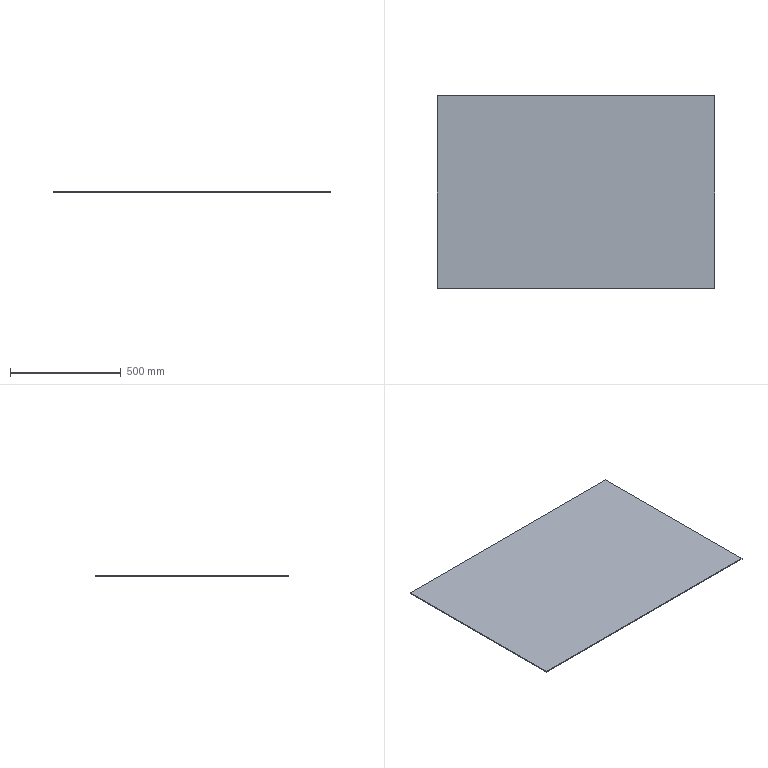Part | STEP file | 08-Middle cover plate | 1 solid | 6 faces | box 1252 x 870 x 4 mm | volume 4356960 mm3 | plane 6
STEP:
#1=CARTESIAN_POINT('',(0.,0.,0.));
#2=DIRECTION('',(0.,0.,1.));
#3=DIRECTION('',(1.,0.,0.));
#4=AXIS2_PLACEMENT_3D('',#1,#2,#3);
#5=CARTESIAN_POINT('',(0.,0.,0.));
#6=VERTEX_POINT('',#5);
#7=CARTESIAN_POINT('',(0.,-870.,0.));
#8=VERTEX_POINT('',#7);
#9=CARTESIAN_POINT('',(0.,0.,0.));
#10=DIRECTION('',(0.,-1.,0.));
#11=VECTOR('',#10,1.);
#12=LINE('',#9,#11);
#13=CARTESIAN_POINT('',(0.,0.,4.));
#14=DIRECTION('',(1.,0.,0.));
#15=DIRECTION('',(0.,1.,0.));
#16=AXIS2_PLACEMENT_3D('',#13,#14,#15);
#17=PLANE('',#16);
#18=CARTESIAN_POINT('',(0.,-4.));
#19=DIRECTION('',(-1.,0.));
#20=VECTOR('',#19,1.);
#21=LINE('',#18,#20);
#22=(GEOMETRIC_REPRESENTATION_CONTEXT(2)PARAMETRIC_REPRESENTATION_CONTEXT()REPRESENTATION_CONTEXT('',''));
#23=DEFINITIONAL_REPRESENTATION('',(#21),#22);
#24=PCURVE('',#17,#23);
#25=CARTESIAN_POINT('',(0.,0.,0.));
#26=DIRECTION('',(0.,0.,1.));
#27=DIRECTION('',(1.,0.,0.));
#28=AXIS2_PLACEMENT_3D('',#25,#26,#27);
#29=PLANE('',#28);
#30=CARTESIAN_POINT('',(0.,0.));
#31=DIRECTION('',(0.,-1.));
#32=VECTOR('',#31,1.);
#33=LINE('',#30,#32);
#34=(GEOMETRIC_REPRESENTATION_CONTEXT(2)PARAMETRIC_REPRESENTATION_CONTEXT()REPRESENTATION_CONTEXT('',''));
#35=DEFINITIONAL_REPRESENTATION('',(#33),#34);
#36=PCURVE('',#29,#35);
#37=SURFACE_CURVE('',#12,(#24,#36),.PCURVE_S1.);
#38=EDGE_CURVE('',#6,#8,#37,.T.);
#39=ORIENTED_EDGE('',*,*,#38,.T.);
#40=CARTESIAN_POINT('',(0.,-870.,4.));
#41=VERTEX_POINT('',#40);
#42=CARTESIAN_POINT('',(0.,-870.,4.));
#43=DIRECTION('',(0.,0.,-1.));
#44=VECTOR('',#43,1.);
#45=LINE('',#42,#44);
#46=CARTESIAN_POINT('',(-870.,0.));
#47=DIRECTION('',(0.,-1.));
#48=VECTOR('',#47,1.);
#49=LINE('',#46,#48);
#50=(GEOMETRIC_REPRESENTATION_CONTEXT(2)PARAMETRIC_REPRESENTATION_CONTEXT()REPRESENTATION_CONTEXT('',''));
#51=DEFINITIONAL_REPRESENTATION('',(#49),#50);
#52=PCURVE('',#17,#51);
#53=CARTESIAN_POINT('',(0.,-870.,4.));
#54=DIRECTION('',(0.,1.,0.));
#55=DIRECTION('',(0.,0.,1.));
#56=AXIS2_PLACEMENT_3D('',#53,#54,#55);
#57=PLANE('',#56);
#58=CARTESIAN_POINT('',(0.,0.));
#59=DIRECTION('',(-1.,0.));
#60=VECTOR('',#59,1.);
#61=LINE('',#58,#60);
#62=(GEOMETRIC_REPRESENTATION_CONTEXT(2)PARAMETRIC_REPRESENTATION_CONTEXT()REPRESENTATION_CONTEXT('',''));
#63=DEFINITIONAL_REPRESENTATION('',(#61),#62);
#64=PCURVE('',#57,#63);
#65=SURFACE_CURVE('',#45,(#52,#64),.PCURVE_S1.);
#66=EDGE_CURVE('',#41,#8,#65,.T.);
#67=ORIENTED_EDGE('',*,*,#66,.F.);
#68=CARTESIAN_POINT('',(0.,0.,4.));
#69=VERTEX_POINT('',#68);
#70=CARTESIAN_POINT('',(0.,0.,4.));
#71=DIRECTION('',(0.,-1.,0.));
#72=VECTOR('',#71,1.);
#73=LINE('',#70,#72);
#74=CARTESIAN_POINT('',(0.,0.));
#75=DIRECTION('',(-1.,0.));
#76=VECTOR('',#75,1.);
#77=LINE('',#74,#76);
#78=(GEOMETRIC_REPRESENTATION_CONTEXT(2)PARAMETRIC_REPRESENTATION_CONTEXT()REPRESENTATION_CONTEXT('',''));
#79=DEFINITIONAL_REPRESENTATION('',(#77),#78);
#80=PCURVE('',#17,#79);
#81=CARTESIAN_POINT('',(0.,0.,4.));
#82=DIRECTION('',(0.,0.,1.));
#83=DIRECTION('',(1.,0.,0.));
#84=AXIS2_PLACEMENT_3D('',#81,#82,#83);
#85=PLANE('',#84);
#86=CARTESIAN_POINT('',(0.,0.));
#87=DIRECTION('',(0.,-1.));
#88=VECTOR('',#87,1.);
#89=LINE('',#86,#88);
#90=(GEOMETRIC_REPRESENTATION_CONTEXT(2)PARAMETRIC_REPRESENTATION_CONTEXT()REPRESENTATION_CONTEXT('',''));
#91=DEFINITIONAL_REPRESENTATION('',(#89),#90);
#92=PCURVE('',#85,#91);
#93=SURFACE_CURVE('',#73,(#80,#92),.PCURVE_S1.);
#94=EDGE_CURVE('',#69,#41,#93,.T.);
#95=ORIENTED_EDGE('',*,*,#94,.F.);
#96=CARTESIAN_POINT('',(0.,0.,4.));
#97=DIRECTION('',(0.,0.,-1.));
#98=VECTOR('',#97,1.);
#99=LINE('',#96,#98);
#100=CARTESIAN_POINT('',(0.,0.));
#101=DIRECTION('',(0.,-1.));
#102=VECTOR('',#101,1.);
#103=LINE('',#100,#102);
#104=(GEOMETRIC_REPRESENTATION_CONTEXT(2)PARAMETRIC_REPRESENTATION_CONTEXT()REPRESENTATION_CONTEXT('',''));
#105=DEFINITIONAL_REPRESENTATION('',(#103),#104);
#106=PCURVE('',#17,#105);
#107=CARTESIAN_POINT('',(0.,0.,4.));
#108=DIRECTION('',(0.,-1.,0.));
#109=DIRECTION('',(0.,0.,-1.));
#110=AXIS2_PLACEMENT_3D('',#107,#108,#109);
#111=PLANE('',#110);
#112=CARTESIAN_POINT('',(0.,0.));
#113=DIRECTION('',(1.,0.));
#114=VECTOR('',#113,1.);
#115=LINE('',#112,#114);
#116=(GEOMETRIC_REPRESENTATION_CONTEXT(2)PARAMETRIC_REPRESENTATION_CONTEXT()REPRESENTATION_CONTEXT('',''));
#117=DEFINITIONAL_REPRESENTATION('',(#115),#116);
#118=PCURVE('',#111,#117);
#119=SURFACE_CURVE('',#99,(#106,#118),.PCURVE_S1.);
#120=EDGE_CURVE('',#69,#6,#119,.T.);
#121=ORIENTED_EDGE('',*,*,#120,.T.);
#122=EDGE_LOOP('',(#39,#67,#95,#121));
#123=FACE_BOUND('',#122,.T.);
#124=ADVANCED_FACE('',(#123),#17,.F.);
#125=CARTESIAN_POINT('',(1252.,-870.,0.));
#126=VERTEX_POINT('',#125);
#127=CARTESIAN_POINT('',(0.,-870.,0.));
#128=DIRECTION('',(1.,0.,0.));
#129=VECTOR('',#128,1.);
#130=LINE('',#127,#129);
#131=CARTESIAN_POINT('',(-4.,0.));
#132=DIRECTION('',(0.,1.));
#133=VECTOR('',#132,1.);
#134=LINE('',#131,#133);
#135=(GEOMETRIC_REPRESENTATION_CONTEXT(2)PARAMETRIC_REPRESENTATION_CONTEXT()REPRESENTATION_CONTEXT('',''));
#136=DEFINITIONAL_REPRESENTATION('',(#134),#135);
#137=PCURVE('',#57,#136);
#138=CARTESIAN_POINT('',(0.,-870.));
#139=DIRECTION('',(1.,0.));
#140=VECTOR('',#139,1.);
#141=LINE('',#138,#140);
#142=(GEOMETRIC_REPRESENTATION_CONTEXT(2)PARAMETRIC_REPRESENTATION_CONTEXT()REPRESENTATION_CONTEXT('',''));
#143=DEFINITIONAL_REPRESENTATION('',(#141),#142);
#144=PCURVE('',#29,#143);
#145=SURFACE_CURVE('',#130,(#137,#144),.PCURVE_S1.);
#146=EDGE_CURVE('',#8,#126,#145,.T.);
#147=ORIENTED_EDGE('',*,*,#146,.T.);
#148=CARTESIAN_POINT('',(1252.,-870.,4.));
#149=VERTEX_POINT('',#148);
#150=CARTESIAN_POINT('',(1252.,-870.,4.));
#151=DIRECTION('',(0.,0.,-1.));
#152=VECTOR('',#151,1.);
#153=LINE('',#150,#152);
#154=CARTESIAN_POINT('',(0.,1252.));
#155=DIRECTION('',(-1.,0.));
#156=VECTOR('',#155,1.);
#157=LINE('',#154,#156);
#158=(GEOMETRIC_REPRESENTATION_CONTEXT(2)PARAMETRIC_REPRESENTATION_CONTEXT()REPRESENTATION_CONTEXT('',''));
#159=DEFINITIONAL_REPRESENTATION('',(#157),#158);
#160=PCURVE('',#57,#159);
#161=CARTESIAN_POINT('',(1252.,0.,4.));
#162=DIRECTION('',(-1.,0.,0.));
#163=DIRECTION('',(0.,0.,1.));
#164=AXIS2_PLACEMENT_3D('',#161,#162,#163);
#165=PLANE('',#164);
#166=CARTESIAN_POINT('',(0.,-870.));
#167=DIRECTION('',(-1.,0.));
#168=VECTOR('',#167,1.);
#169=LINE('',#166,#168);
#170=(GEOMETRIC_REPRESENTATION_CONTEXT(2)PARAMETRIC_REPRESENTATION_CONTEXT()REPRESENTATION_CONTEXT('',''));
#171=DEFINITIONAL_REPRESENTATION('',(#169),#170);
#172=PCURVE('',#165,#171);
#173=SURFACE_CURVE('',#153,(#160,#172),.PCURVE_S1.);
#174=EDGE_CURVE('',#149,#126,#173,.T.);
#175=ORIENTED_EDGE('',*,*,#174,.F.);
#176=CARTESIAN_POINT('',(0.,-870.,4.));
#177=DIRECTION('',(1.,0.,0.));
#178=VECTOR('',#177,1.);
#179=LINE('',#176,#178);
#180=CARTESIAN_POINT('',(0.,0.));
#181=DIRECTION('',(0.,1.));
#182=VECTOR('',#181,1.);
#183=LINE('',#180,#182);
#184=(GEOMETRIC_REPRESENTATION_CONTEXT(2)PARAMETRIC_REPRESENTATION_CONTEXT()REPRESENTATION_CONTEXT('',''));
#185=DEFINITIONAL_REPRESENTATION('',(#183),#184);
#186=PCURVE('',#57,#185);
#187=CARTESIAN_POINT('',(0.,-870.));
#188=DIRECTION('',(1.,0.));
#189=VECTOR('',#188,1.);
#190=LINE('',#187,#189);
#191=(GEOMETRIC_REPRESENTATION_CONTEXT(2)PARAMETRIC_REPRESENTATION_CONTEXT()REPRESENTATION_CONTEXT('',''));
#192=DEFINITIONAL_REPRESENTATION('',(#190),#191);
#193=PCURVE('',#85,#192);
#194=SURFACE_CURVE('',#179,(#186,#193),.PCURVE_S1.);
#195=EDGE_CURVE('',#41,#149,#194,.T.);
#196=ORIENTED_EDGE('',*,*,#195,.F.);
#197=ORIENTED_EDGE('',*,*,#66,.T.);
#198=EDGE_LOOP('',(#147,#175,#196,#197));
#199=FACE_BOUND('',#198,.T.);
#200=ADVANCED_FACE('',(#199),#57,.F.);
#201=CARTESIAN_POINT('',(1252.,0.,0.));
#202=VERTEX_POINT('',#201);
#203=CARTESIAN_POINT('',(1252.,0.,0.));
#204=DIRECTION('',(0.,1.,0.));
#205=VECTOR('',#204,1.);
#206=LINE('',#203,#205);
#207=CARTESIAN_POINT('',(-4.,0.));
#208=DIRECTION('',(0.,1.));
#209=VECTOR('',#208,1.);
#210=LINE('',#207,#209);
#211=(GEOMETRIC_REPRESENTATION_CONTEXT(2)PARAMETRIC_REPRESENTATION_CONTEXT()REPRESENTATION_CONTEXT('',''));
#212=DEFINITIONAL_REPRESENTATION('',(#210),#211);
#213=PCURVE('',#165,#212);
#214=CARTESIAN_POINT('',(1252.,0.));
#215=DIRECTION('',(0.,1.));
#216=VECTOR('',#215,1.);
#217=LINE('',#214,#216);
#218=(GEOMETRIC_REPRESENTATION_CONTEXT(2)PARAMETRIC_REPRESENTATION_CONTEXT()REPRESENTATION_CONTEXT('',''));
#219=DEFINITIONAL_REPRESENTATION('',(#217),#218);
#220=PCURVE('',#29,#219);
#221=SURFACE_CURVE('',#206,(#213,#220),.PCURVE_S1.);
#222=EDGE_CURVE('',#126,#202,#221,.T.);
#223=ORIENTED_EDGE('',*,*,#222,.T.);
#224=CARTESIAN_POINT('',(1252.,0.,4.));
#225=VERTEX_POINT('',#224);
#226=CARTESIAN_POINT('',(1252.,0.,4.));
#227=DIRECTION('',(0.,0.,-1.));
#228=VECTOR('',#227,1.);
#229=LINE('',#226,#228);
#230=CARTESIAN_POINT('',(0.,0.));
#231=DIRECTION('',(-1.,0.));
#232=VECTOR('',#231,1.);
#233=LINE('',#230,#232);
#234=(GEOMETRIC_REPRESENTATION_CONTEXT(2)PARAMETRIC_REPRESENTATION_CONTEXT()REPRESENTATION_CONTEXT('',''));
#235=DEFINITIONAL_REPRESENTATION('',(#233),#234);
#236=PCURVE('',#165,#235);
#237=CARTESIAN_POINT('',(0.,1252.));
#238=DIRECTION('',(1.,0.));
#239=VECTOR('',#238,1.);
#240=LINE('',#237,#239);
#241=(GEOMETRIC_REPRESENTATION_CONTEXT(2)PARAMETRIC_REPRESENTATION_CONTEXT()REPRESENTATION_CONTEXT('',''));
#242=DEFINITIONAL_REPRESENTATION('',(#240),#241);
#243=PCURVE('',#111,#242);
#244=SURFACE_CURVE('',#229,(#236,#243),.PCURVE_S1.);
#245=EDGE_CURVE('',#225,#202,#244,.T.);
#246=ORIENTED_EDGE('',*,*,#245,.F.);
#247=CARTESIAN_POINT('',(1252.,0.,4.));
#248=DIRECTION('',(0.,1.,0.));
#249=VECTOR('',#248,1.);
#250=LINE('',#247,#249);
#251=CARTESIAN_POINT('',(0.,0.));
#252=DIRECTION('',(0.,1.));
#253=VECTOR('',#252,1.);
#254=LINE('',#251,#253);
#255=(GEOMETRIC_REPRESENTATION_CONTEXT(2)PARAMETRIC_REPRESENTATION_CONTEXT()REPRESENTATION_CONTEXT('',''));
#256=DEFINITIONAL_REPRESENTATION('',(#254),#255);
#257=PCURVE('',#165,#256);
#258=CARTESIAN_POINT('',(1252.,0.));
#259=DIRECTION('',(0.,1.));
#260=VECTOR('',#259,1.);
#261=LINE('',#258,#260);
#262=(GEOMETRIC_REPRESENTATION_CONTEXT(2)PARAMETRIC_REPRESENTATION_CONTEXT()REPRESENTATION_CONTEXT('',''));
#263=DEFINITIONAL_REPRESENTATION('',(#261),#262);
#264=PCURVE('',#85,#263);
#265=SURFACE_CURVE('',#250,(#257,#264),.PCURVE_S1.);
#266=EDGE_CURVE('',#149,#225,#265,.T.);
#267=ORIENTED_EDGE('',*,*,#266,.F.);
#268=ORIENTED_EDGE('',*,*,#174,.T.);
#269=EDGE_LOOP('',(#223,#246,#267,#268));
#270=FACE_BOUND('',#269,.T.);
#271=ADVANCED_FACE('',(#270),#165,.F.);
#272=CARTESIAN_POINT('',(0.,0.,0.));
#273=DIRECTION('',(-1.,0.,0.));
#274=VECTOR('',#273,1.);
#275=LINE('',#272,#274);
#276=CARTESIAN_POINT('',(4.,0.));
#277=DIRECTION('',(0.,-1.));
#278=VECTOR('',#277,1.);
#279=LINE('',#276,#278);
#280=(GEOMETRIC_REPRESENTATION_CONTEXT(2)PARAMETRIC_REPRESENTATION_CONTEXT()REPRESENTATION_CONTEXT('',''));
#281=DEFINITIONAL_REPRESENTATION('',(#279),#280);
#282=PCURVE('',#111,#281);
#283=CARTESIAN_POINT('',(0.,0.));
#284=DIRECTION('',(-1.,0.));
#285=VECTOR('',#284,1.);
#286=LINE('',#283,#285);
#287=(GEOMETRIC_REPRESENTATION_CONTEXT(2)PARAMETRIC_REPRESENTATION_CONTEXT()REPRESENTATION_CONTEXT('',''));
#288=DEFINITIONAL_REPRESENTATION('',(#286),#287);
#289=PCURVE('',#29,#288);
#290=SURFACE_CURVE('',#275,(#282,#289),.PCURVE_S1.);
#291=EDGE_CURVE('',#202,#6,#290,.T.);
#292=ORIENTED_EDGE('',*,*,#291,.T.);
#293=ORIENTED_EDGE('',*,*,#120,.F.);
#294=CARTESIAN_POINT('',(0.,0.,4.));
#295=DIRECTION('',(-1.,0.,0.));
#296=VECTOR('',#295,1.);
#297=LINE('',#294,#296);
#298=CARTESIAN_POINT('',(0.,0.));
#299=DIRECTION('',(0.,-1.));
#300=VECTOR('',#299,1.);
#301=LINE('',#298,#300);
#302=(GEOMETRIC_REPRESENTATION_CONTEXT(2)PARAMETRIC_REPRESENTATION_CONTEXT()REPRESENTATION_CONTEXT('',''));
#303=DEFINITIONAL_REPRESENTATION('',(#301),#302);
#304=PCURVE('',#111,#303);
#305=CARTESIAN_POINT('',(0.,0.));
#306=DIRECTION('',(-1.,0.));
#307=VECTOR('',#306,1.);
#308=LINE('',#305,#307);
#309=(GEOMETRIC_REPRESENTATION_CONTEXT(2)PARAMETRIC_REPRESENTATION_CONTEXT()REPRESENTATION_CONTEXT('',''));
#310=DEFINITIONAL_REPRESENTATION('',(#308),#309);
#311=PCURVE('',#85,#310);
#312=SURFACE_CURVE('',#297,(#304,#311),.PCURVE_S1.);
#313=EDGE_CURVE('',#225,#69,#312,.T.);
#314=ORIENTED_EDGE('',*,*,#313,.F.);
#315=ORIENTED_EDGE('',*,*,#245,.T.);
#316=EDGE_LOOP('',(#292,#293,#314,#315));
#317=FACE_BOUND('',#316,.T.);
#318=ADVANCED_FACE('',(#317),#111,.F.);
#319=ORIENTED_EDGE('',*,*,#94,.T.);
#320=ORIENTED_EDGE('',*,*,#195,.T.);
#321=ORIENTED_EDGE('',*,*,#266,.T.);
#322=ORIENTED_EDGE('',*,*,#313,.T.);
#323=EDGE_LOOP('',(#319,#320,#321,#322));
#324=FACE_BOUND('',#323,.T.);
#325=ADVANCED_FACE('',(#324),#85,.T.);
#326=ORIENTED_EDGE('',*,*,#38,.F.);
#327=ORIENTED_EDGE('',*,*,#291,.F.);
#328=ORIENTED_EDGE('',*,*,#222,.F.);
#329=ORIENTED_EDGE('',*,*,#146,.F.);
#330=EDGE_LOOP('',(#326,#327,#328,#329));
#331=FACE_BOUND('',#330,.T.);
#332=ADVANCED_FACE('',(#331),#29,.F.);
#333=CLOSED_SHELL('',(#124,#200,#271,#318,#325,#332));
#334=MANIFOLD_SOLID_BREP('',#333);
#335=(LENGTH_UNIT()NAMED_UNIT(*)SI_UNIT(.MILLI.,.METRE.));
#336=UNCERTAINTY_MEASURE_WITH_UNIT(LENGTH_MEASURE(0.0000001),#335,'','');
#337=(NAMED_UNIT(*)PLANE_ANGLE_UNIT()SI_UNIT($,.RADIAN.));
#338=(NAMED_UNIT(*)SI_UNIT($,.STERADIAN.)SOLID_ANGLE_UNIT());
#339=(GEOMETRIC_REPRESENTATION_CONTEXT(3)GLOBAL_UNCERTAINTY_ASSIGNED_CONTEXT((#336))GLOBAL_UNIT_ASSIGNED_CONTEXT((#335,#337,#338))REPRESENTATION_CONTEXT('',''));
#340=ADVANCED_BREP_SHAPE_REPRESENTATION('',(#4,#334),#339);